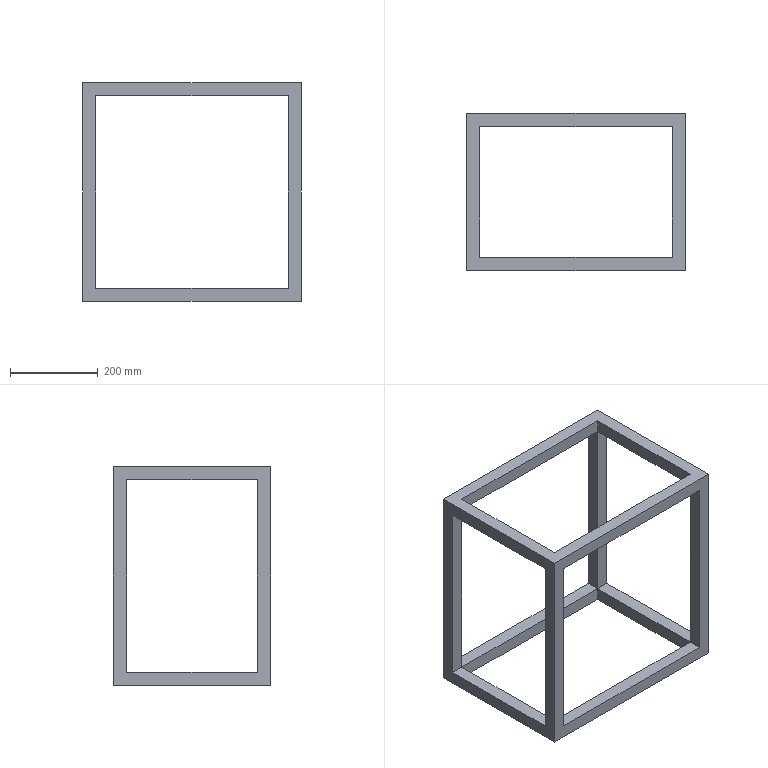Part | STEP file | 1 solid | 30 faces | box 498.959 x 359.164 x 500 mm | volume 4457242 mm3 | plane 30